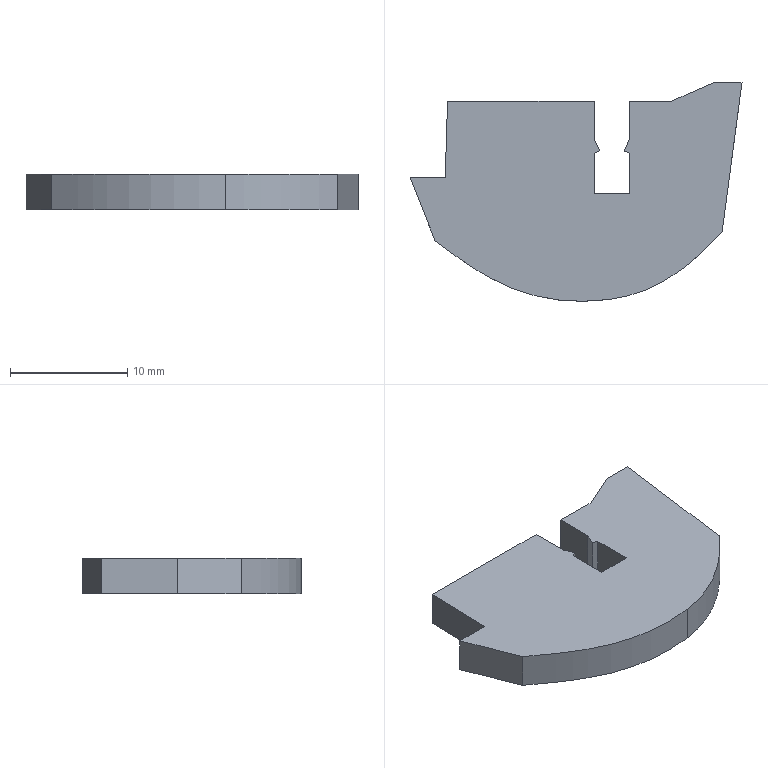Part | SolidWorks | features BaseBody 1 | 1 solid | 21 faces | box 28.291 x 18.638 x 3 mm | volume 1097 mm3 | plane 15 | spline 6
STEP:
#1=CARTESIAN_POINT('',(9.111,-14.247,-1.5));
#2=VERTEX_POINT('',#1);
#3=CARTESIAN_POINT('',(-0.4619,-19.968,-1.5));
#4=VERTEX_POINT('',#3);
#5=CARTESIAN_POINT('',(9.111,-14.247,-1.5));
#6=CARTESIAN_POINT('',(7.044,-16.596,-1.5));
#7=CARTESIAN_POINT('',(3.804,-19.425,-1.5));
#8=CARTESIAN_POINT('',(-0.4619,-19.968,-1.5));
#9=B_SPLINE_CURVE_WITH_KNOTS('',3,(#5,#6,#7,#8),.UNSPECIFIED.,.F.,.F.,(4,4),(0.9,1.),.UNSPECIFIED.);
#10=EDGE_CURVE('',#2,#4,#9,.T.);
#11=ORIENTED_EDGE('',*,*,#10,.T.);
#12=CARTESIAN_POINT('',(-15.322,-15.,-1.5));
#13=VERTEX_POINT('',#12);
#14=CARTESIAN_POINT('',(-0.4619,-19.968,-1.5));
#15=CARTESIAN_POINT('',(-7.402,-20.85,-1.5));
#16=CARTESIAN_POINT('',(-11.363,-17.925,-1.5));
#17=CARTESIAN_POINT('',(-15.322,-15.,-1.5));
#18=B_SPLINE_CURVE_WITH_KNOTS('',3,(#14,#15,#16,#17),.UNSPECIFIED.,.F.,.F.,(4,4),(0.,0.05),.UNSPECIFIED.);
#19=EDGE_CURVE('',#4,#13,#18,.T.);
#20=ORIENTED_EDGE('',*,*,#19,.T.);
#21=CARTESIAN_POINT('',(-17.475,-9.564,-1.5));
#22=VERTEX_POINT('',#21);
#23=CARTESIAN_POINT('',(-15.322,-15.,-1.5));
#24=CARTESIAN_POINT('',(-16.041,-13.188,-1.5));
#25=CARTESIAN_POINT('',(-16.758,-11.376,-1.5));
#26=CARTESIAN_POINT('',(-17.475,-9.564,-1.5));
#27=B_SPLINE_CURVE_WITH_KNOTS('',3,(#23,#24,#25,#26),.UNSPECIFIED.,.F.,.F.,(4,4),(0.05,0.1),.UNSPECIFIED.);
#28=EDGE_CURVE('',#13,#22,#27,.T.);
#29=ORIENTED_EDGE('',*,*,#28,.T.);
#30=CARTESIAN_POINT('',(-14.475,-9.564,-1.5));
#31=VERTEX_POINT('',#30);
#32=CARTESIAN_POINT('',(-17.475,-9.564,-1.5));
#33=DIRECTION('',(1.,0.,0.));
#34=VECTOR('',#33,1000.);
#35=LINE('',#32,#34);
#36=EDGE_CURVE('',#22,#31,#35,.T.);
#37=ORIENTED_EDGE('',*,*,#36,.T.);
#38=CARTESIAN_POINT('',(-14.277,-3.061,-1.5));
#39=VERTEX_POINT('',#38);
#40=CARTESIAN_POINT('',(-14.475,-9.564,-1.5));
#41=CARTESIAN_POINT('',(-14.393,-6.871,-1.5));
#42=CARTESIAN_POINT('',(-14.359,-5.755,-1.5));
#43=CARTESIAN_POINT('',(-14.277,-3.061,-1.5));
#44=B_SPLINE_CURVE_WITH_KNOTS('',3,(#40,#41,#42,#43),.UNSPECIFIED.,.F.,.F.,(4,4),(0.15,0.2),.UNSPECIFIED.);
#45=EDGE_CURVE('',#31,#39,#44,.T.);
#46=ORIENTED_EDGE('',*,*,#45,.T.);
#47=CARTESIAN_POINT('',(-1.772,-3.061,-1.5));
#48=VERTEX_POINT('',#47);
#49=CARTESIAN_POINT('',(-14.277,-3.061,-1.5));
#50=DIRECTION('',(1.,0.,0.));
#51=VECTOR('',#50,1000.);
#52=LINE('',#49,#51);
#53=EDGE_CURVE('',#39,#48,#52,.T.);
#54=ORIENTED_EDGE('',*,*,#53,.T.);
#55=CARTESIAN_POINT('',(-1.772,-6.322,-1.5));
#56=VERTEX_POINT('',#55);
#57=CARTESIAN_POINT('',(-1.772,-3.061,-1.5));
#58=DIRECTION('',(0.,-1.,0.));
#59=VECTOR('',#58,1000.);
#60=LINE('',#57,#59);
#61=EDGE_CURVE('',#48,#56,#60,.T.);
#62=ORIENTED_EDGE('',*,*,#61,.T.);
#63=CARTESIAN_POINT('',(-1.323,-7.28,-1.5));
#64=VERTEX_POINT('',#63);
#65=CARTESIAN_POINT('',(-1.772,-6.322,-1.5));
#66=DIRECTION('',(0.4242,-0.9056,0.));
#67=VECTOR('',#66,1000.);
#68=LINE('',#65,#67);
#69=EDGE_CURVE('',#56,#64,#68,.T.);
#70=ORIENTED_EDGE('',*,*,#69,.T.);
#71=CARTESIAN_POINT('',(-1.772,-7.511,-1.5));
#72=VERTEX_POINT('',#71);
#73=CARTESIAN_POINT('',(-1.323,-7.28,-1.5));
#74=DIRECTION('',(-0.8893,-0.4572,0.));
#75=VECTOR('',#74,1000.);
#76=LINE('',#73,#75);
#77=EDGE_CURVE('',#64,#72,#76,.T.);
#78=ORIENTED_EDGE('',*,*,#77,.T.);
#79=CARTESIAN_POINT('',(-1.772,-10.963,-1.5));
#80=VERTEX_POINT('',#79);
#81=CARTESIAN_POINT('',(-1.772,-7.511,-1.5));
#82=DIRECTION('',(0.,-1.,0.));
#83=VECTOR('',#82,1000.);
#84=LINE('',#81,#83);
#85=EDGE_CURVE('',#72,#80,#84,.T.);
#86=ORIENTED_EDGE('',*,*,#85,.T.);
#87=CARTESIAN_POINT('',(1.224,-10.963,-1.5));
#88=VERTEX_POINT('',#87);
#89=CARTESIAN_POINT('',(-1.772,-10.963,-1.5));
#90=DIRECTION('',(1.,0.,0.));
#91=VECTOR('',#90,1000.);
#92=LINE('',#89,#91);
#93=EDGE_CURVE('',#80,#88,#92,.T.);
#94=ORIENTED_EDGE('',*,*,#93,.T.);
#95=CARTESIAN_POINT('',(1.224,-7.511,-1.5));
#96=VERTEX_POINT('',#95);
#97=CARTESIAN_POINT('',(1.224,-10.963,-1.5));
#98=DIRECTION('',(0.,1.,0.));
#99=VECTOR('',#98,1000.);
#100=LINE('',#97,#99);
#101=EDGE_CURVE('',#88,#96,#100,.T.);
#102=ORIENTED_EDGE('',*,*,#101,.T.);
#103=CARTESIAN_POINT('',(0.7738,-7.315,-1.5));
#104=VERTEX_POINT('',#103);
#105=CARTESIAN_POINT('',(1.224,-7.511,-1.5));
#106=DIRECTION('',(-0.917,0.3989,0.));
#107=VECTOR('',#106,1000.);
#108=LINE('',#105,#107);
#109=EDGE_CURVE('',#96,#104,#108,.T.);
#110=ORIENTED_EDGE('',*,*,#109,.T.);
#111=CARTESIAN_POINT('',(1.224,-6.304,-1.5));
#112=VERTEX_POINT('',#111);
#113=CARTESIAN_POINT('',(0.7738,-7.315,-1.5));
#114=DIRECTION('',(0.4071,0.9134,0.));
#115=VECTOR('',#114,1000.);
#116=LINE('',#113,#115);
#117=EDGE_CURVE('',#104,#112,#116,.T.);
#118=ORIENTED_EDGE('',*,*,#117,.T.);
#119=CARTESIAN_POINT('',(1.224,-3.061,-1.5));
#120=VERTEX_POINT('',#119);
#121=CARTESIAN_POINT('',(1.224,-6.304,-1.5));
#122=DIRECTION('',(0.,1.,0.));
#123=VECTOR('',#122,1000.);
#124=LINE('',#121,#123);
#125=EDGE_CURVE('',#112,#120,#124,.T.);
#126=ORIENTED_EDGE('',*,*,#125,.T.);
#127=CARTESIAN_POINT('',(4.844,-3.061,-1.5));
#128=VERTEX_POINT('',#127);
#129=CARTESIAN_POINT('',(1.224,-3.061,-1.5));
#130=DIRECTION('',(1.,0.,0.));
#131=VECTOR('',#130,1000.);
#132=LINE('',#129,#131);
#133=EDGE_CURVE('',#120,#128,#132,.T.);
#134=ORIENTED_EDGE('',*,*,#133,.T.);
#135=CARTESIAN_POINT('',(8.366,-1.493,-1.5));
#136=VERTEX_POINT('',#135);
#137=CARTESIAN_POINT('',(4.844,-3.061,-1.5));
#138=DIRECTION('',(0.9136,0.4066,0.));
#139=VECTOR('',#138,1000.);
#140=LINE('',#137,#139);
#141=EDGE_CURVE('',#128,#136,#140,.T.);
#142=ORIENTED_EDGE('',*,*,#141,.T.);
#143=CARTESIAN_POINT('',(10.816,-1.489,-1.5));
#144=VERTEX_POINT('',#143);
#145=CARTESIAN_POINT('',(8.366,-1.493,-1.5));
#146=CARTESIAN_POINT('',(9.409,-1.491,-1.5));
#147=CARTESIAN_POINT('',(10.816,-1.489,-1.5));
#148=B_SPLINE_CURVE_WITH_KNOTS('',2,(#145,#146,#147),.UNSPECIFIED.,.F.,.F.,(3,3),(0.8,0.85),.UNSPECIFIED.);
#149=EDGE_CURVE('',#136,#144,#148,.T.);
#150=ORIENTED_EDGE('',*,*,#149,.T.);
#151=CARTESIAN_POINT('',(10.816,-1.489,-1.5));
#152=CARTESIAN_POINT('',(10.53,-3.621,-1.5));
#153=CARTESIAN_POINT('',(9.723,-9.669,-1.5));
#154=CARTESIAN_POINT('',(9.111,-14.247,-1.5));
#155=B_SPLINE_CURVE_WITH_KNOTS('',3,(#151,#152,#153,#154),.UNSPECIFIED.,.F.,.F.,(4,4),(0.85,0.9),.UNSPECIFIED.);
#156=EDGE_CURVE('',#144,#2,#155,.T.);
#157=ORIENTED_EDGE('',*,*,#156,.T.);
#158=EDGE_LOOP('',(#11,#20,#29,#37,#46,#54,#62,#70,#78,#86,#94,#102,#110,#118,#126,#134,#142,#150,#157));
#159=FACE_OUTER_BOUND('',#158,.T.);
#160=CARTESIAN_POINT('',(5.149,-17.785,-1.5));
#161=DIRECTION('',(0.,0.,1.));
#162=DIRECTION('',(1.,0.,0.));
#163=AXIS2_PLACEMENT_3D('',#160,#161,#162);
#164=PLANE('',#163);
#165=ADVANCED_FACE('',(#159),#164,.F.);
#166=CARTESIAN_POINT('',(9.111,-14.247,1.5));
#167=VERTEX_POINT('',#166);
#168=CARTESIAN_POINT('',(-0.4619,-19.968,1.5));
#169=VERTEX_POINT('',#168);
#170=CARTESIAN_POINT('',(9.111,-14.247,1.5));
#171=CARTESIAN_POINT('',(7.044,-16.596,1.5));
#172=CARTESIAN_POINT('',(3.804,-19.425,1.5));
#173=CARTESIAN_POINT('',(-0.4619,-19.968,1.5));
#174=B_SPLINE_CURVE_WITH_KNOTS('',3,(#170,#171,#172,#173),.UNSPECIFIED.,.F.,.F.,(4,4),(0.9,1.),.UNSPECIFIED.);
#175=EDGE_CURVE('',#167,#169,#174,.T.);
#176=ORIENTED_EDGE('',*,*,#175,.F.);
#177=CARTESIAN_POINT('',(10.816,-1.489,1.5));
#178=VERTEX_POINT('',#177);
#179=CARTESIAN_POINT('',(10.816,-1.489,1.5));
#180=CARTESIAN_POINT('',(10.53,-3.621,1.5));
#181=CARTESIAN_POINT('',(9.723,-9.669,1.5));
#182=CARTESIAN_POINT('',(9.111,-14.247,1.5));
#183=B_SPLINE_CURVE_WITH_KNOTS('',3,(#179,#180,#181,#182),.UNSPECIFIED.,.F.,.F.,(4,4),(0.85,0.9),.UNSPECIFIED.);
#184=EDGE_CURVE('',#178,#167,#183,.T.);
#185=ORIENTED_EDGE('',*,*,#184,.F.);
#186=CARTESIAN_POINT('',(8.366,-1.493,1.5));
#187=VERTEX_POINT('',#186);
#188=CARTESIAN_POINT('',(8.366,-1.493,1.5));
#189=CARTESIAN_POINT('',(9.409,-1.491,1.5));
#190=CARTESIAN_POINT('',(10.816,-1.489,1.5));
#191=B_SPLINE_CURVE_WITH_KNOTS('',2,(#188,#189,#190),.UNSPECIFIED.,.F.,.F.,(3,3),(0.8,0.85),.UNSPECIFIED.);
#192=EDGE_CURVE('',#187,#178,#191,.T.);
#193=ORIENTED_EDGE('',*,*,#192,.F.);
#194=CARTESIAN_POINT('',(4.844,-3.061,1.5));
#195=VERTEX_POINT('',#194);
#196=CARTESIAN_POINT('',(4.844,-3.061,1.5));
#197=DIRECTION('',(0.9136,0.4066,0.));
#198=VECTOR('',#197,1000.);
#199=LINE('',#196,#198);
#200=EDGE_CURVE('',#195,#187,#199,.T.);
#201=ORIENTED_EDGE('',*,*,#200,.F.);
#202=CARTESIAN_POINT('',(1.224,-3.061,1.5));
#203=VERTEX_POINT('',#202);
#204=CARTESIAN_POINT('',(1.224,-3.061,1.5));
#205=DIRECTION('',(1.,0.,0.));
#206=VECTOR('',#205,1000.);
#207=LINE('',#204,#206);
#208=EDGE_CURVE('',#203,#195,#207,.T.);
#209=ORIENTED_EDGE('',*,*,#208,.F.);
#210=CARTESIAN_POINT('',(1.224,-6.304,1.5));
#211=VERTEX_POINT('',#210);
#212=CARTESIAN_POINT('',(1.224,-6.304,1.5));
#213=DIRECTION('',(0.,1.,0.));
#214=VECTOR('',#213,1000.);
#215=LINE('',#212,#214);
#216=EDGE_CURVE('',#211,#203,#215,.T.);
#217=ORIENTED_EDGE('',*,*,#216,.F.);
#218=CARTESIAN_POINT('',(0.7738,-7.315,1.5));
#219=VERTEX_POINT('',#218);
#220=CARTESIAN_POINT('',(0.7738,-7.315,1.5));
#221=DIRECTION('',(0.4071,0.9134,0.));
#222=VECTOR('',#221,1000.);
#223=LINE('',#220,#222);
#224=EDGE_CURVE('',#219,#211,#223,.T.);
#225=ORIENTED_EDGE('',*,*,#224,.F.);
#226=CARTESIAN_POINT('',(1.224,-7.511,1.5));
#227=VERTEX_POINT('',#226);
#228=CARTESIAN_POINT('',(1.224,-7.511,1.5));
#229=DIRECTION('',(-0.917,0.3989,0.));
#230=VECTOR('',#229,1000.);
#231=LINE('',#228,#230);
#232=EDGE_CURVE('',#227,#219,#231,.T.);
#233=ORIENTED_EDGE('',*,*,#232,.F.);
#234=CARTESIAN_POINT('',(1.224,-10.963,1.5));
#235=VERTEX_POINT('',#234);
#236=CARTESIAN_POINT('',(1.224,-10.963,1.5));
#237=DIRECTION('',(0.,1.,0.));
#238=VECTOR('',#237,1000.);
#239=LINE('',#236,#238);
#240=EDGE_CURVE('',#235,#227,#239,.T.);
#241=ORIENTED_EDGE('',*,*,#240,.F.);
#242=CARTESIAN_POINT('',(-1.772,-10.963,1.5));
#243=VERTEX_POINT('',#242);
#244=CARTESIAN_POINT('',(-1.772,-10.963,1.5));
#245=DIRECTION('',(1.,0.,0.));
#246=VECTOR('',#245,1000.);
#247=LINE('',#244,#246);
#248=EDGE_CURVE('',#243,#235,#247,.T.);
#249=ORIENTED_EDGE('',*,*,#248,.F.);
#250=CARTESIAN_POINT('',(-1.772,-7.511,1.5));
#251=VERTEX_POINT('',#250);
#252=CARTESIAN_POINT('',(-1.772,-7.511,1.5));
#253=DIRECTION('',(0.,-1.,0.));
#254=VECTOR('',#253,1000.);
#255=LINE('',#252,#254);
#256=EDGE_CURVE('',#251,#243,#255,.T.);
#257=ORIENTED_EDGE('',*,*,#256,.F.);
#258=CARTESIAN_POINT('',(-1.323,-7.28,1.5));
#259=VERTEX_POINT('',#258);
#260=CARTESIAN_POINT('',(-1.323,-7.28,1.5));
#261=DIRECTION('',(-0.8893,-0.4572,0.));
#262=VECTOR('',#261,1000.);
#263=LINE('',#260,#262);
#264=EDGE_CURVE('',#259,#251,#263,.T.);
#265=ORIENTED_EDGE('',*,*,#264,.F.);
#266=CARTESIAN_POINT('',(-1.772,-6.322,1.5));
#267=VERTEX_POINT('',#266);
#268=CARTESIAN_POINT('',(-1.772,-6.322,1.5));
#269=DIRECTION('',(0.4242,-0.9056,0.));
#270=VECTOR('',#269,1000.);
#271=LINE('',#268,#270);
#272=EDGE_CURVE('',#267,#259,#271,.T.);
#273=ORIENTED_EDGE('',*,*,#272,.F.);
#274=CARTESIAN_POINT('',(-1.772,-3.061,1.5));
#275=VERTEX_POINT('',#274);
#276=CARTESIAN_POINT('',(-1.772,-3.061,1.5));
#277=DIRECTION('',(0.,-1.,0.));
#278=VECTOR('',#277,1000.);
#279=LINE('',#276,#278);
#280=EDGE_CURVE('',#275,#267,#279,.T.);
#281=ORIENTED_EDGE('',*,*,#280,.F.);
#282=CARTESIAN_POINT('',(-14.277,-3.061,1.5));
#283=VERTEX_POINT('',#282);
#284=CARTESIAN_POINT('',(-14.277,-3.061,1.5));
#285=DIRECTION('',(1.,0.,0.));
#286=VECTOR('',#285,1000.);
#287=LINE('',#284,#286);
#288=EDGE_CURVE('',#283,#275,#287,.T.);
#289=ORIENTED_EDGE('',*,*,#288,.F.);
#290=CARTESIAN_POINT('',(-14.475,-9.564,1.5));
#291=VERTEX_POINT('',#290);
#292=CARTESIAN_POINT('',(-14.475,-9.564,1.5));
#293=CARTESIAN_POINT('',(-14.393,-6.871,1.5));
#294=CARTESIAN_POINT('',(-14.359,-5.755,1.5));
#295=CARTESIAN_POINT('',(-14.277,-3.061,1.5));
#296=B_SPLINE_CURVE_WITH_KNOTS('',3,(#292,#293,#294,#295),.UNSPECIFIED.,.F.,.F.,(4,4),(0.15,0.2),.UNSPECIFIED.);
#297=EDGE_CURVE('',#291,#283,#296,.T.);
#298=ORIENTED_EDGE('',*,*,#297,.F.);
#299=CARTESIAN_POINT('',(-17.475,-9.564,1.5));
#300=VERTEX_POINT('',#299);
#301=CARTESIAN_POINT('',(-17.475,-9.564,1.5));
#302=DIRECTION('',(1.,0.,0.));
#303=VECTOR('',#302,1000.);
#304=LINE('',#301,#303);
#305=EDGE_CURVE('',#300,#291,#304,.T.);
#306=ORIENTED_EDGE('',*,*,#305,.F.);
#307=CARTESIAN_POINT('',(-15.322,-15.,1.5));
#308=VERTEX_POINT('',#307);
#309=CARTESIAN_POINT('',(-15.322,-15.,1.5));
#310=CARTESIAN_POINT('',(-16.041,-13.188,1.5));
#311=CARTESIAN_POINT('',(-16.758,-11.376,1.5));
#312=CARTESIAN_POINT('',(-17.475,-9.564,1.5));
#313=B_SPLINE_CURVE_WITH_KNOTS('',3,(#309,#310,#311,#312),.UNSPECIFIED.,.F.,.F.,(4,4),(0.05,0.1),.UNSPECIFIED.);
#314=EDGE_CURVE('',#308,#300,#313,.T.);
#315=ORIENTED_EDGE('',*,*,#314,.F.);
#316=CARTESIAN_POINT('',(-0.4619,-19.968,1.5));
#317=CARTESIAN_POINT('',(-7.402,-20.85,1.5));
#318=CARTESIAN_POINT('',(-11.363,-17.925,1.5));
#319=CARTESIAN_POINT('',(-15.322,-15.,1.5));
#320=B_SPLINE_CURVE_WITH_KNOTS('',3,(#316,#317,#318,#319),.UNSPECIFIED.,.F.,.F.,(4,4),(0.,0.05),.UNSPECIFIED.);
#321=EDGE_CURVE('',#169,#308,#320,.T.);
#322=ORIENTED_EDGE('',*,*,#321,.F.);
#323=EDGE_LOOP('',(#176,#185,#193,#201,#209,#217,#225,#233,#241,#249,#257,#265,#273,#281,#289,#298,#306,#315,#322));
#324=FACE_OUTER_BOUND('',#323,.T.);
#325=CARTESIAN_POINT('',(5.149,-17.785,1.5));
#326=DIRECTION('',(0.,0.,1.));
#327=DIRECTION('',(1.,0.,0.));
#328=AXIS2_PLACEMENT_3D('',#325,#326,#327);
#329=PLANE('',#328);
#330=ADVANCED_FACE('',(#324),#329,.T.);
#331=ORIENTED_EDGE('',*,*,#19,.F.);
#332=CARTESIAN_POINT('',(-0.4619,-19.968,1.5));
#333=DIRECTION('',(0.,0.,-1.));
#334=VECTOR('',#333,1000.);
#335=LINE('',#332,#334);
#336=EDGE_CURVE('',#169,#4,#335,.T.);
#337=ORIENTED_EDGE('',*,*,#336,.F.);
#338=ORIENTED_EDGE('',*,*,#321,.T.);
#339=CARTESIAN_POINT('',(-15.322,-15.,1.5));
#340=DIRECTION('',(0.,0.,-1.));
#341=VECTOR('',#340,1000.);
#342=LINE('',#339,#341);
#343=EDGE_CURVE('',#308,#13,#342,.T.);
#344=ORIENTED_EDGE('',*,*,#343,.T.);
#345=EDGE_LOOP('',(#331,#337,#338,#344));
#346=FACE_OUTER_BOUND('',#345,.T.);
#347=CARTESIAN_POINT('',(-0.4619,-19.968,1.5));
#348=CARTESIAN_POINT('',(-0.4619,-19.968,-1.5));
#349=CARTESIAN_POINT('',(-7.402,-20.85,1.5));
#350=CARTESIAN_POINT('',(-7.402,-20.85,-1.5));
#351=CARTESIAN_POINT('',(-11.363,-17.925,1.5));
#352=CARTESIAN_POINT('',(-11.363,-17.925,-1.5));
#353=CARTESIAN_POINT('',(-15.322,-15.,1.5));
#354=CARTESIAN_POINT('',(-15.322,-15.,-1.5));
#355=B_SPLINE_SURFACE_WITH_KNOTS('',3,1,((#347,#348),(#349,#350),(#351,#352),(#353,#354)),.UNSPECIFIED.,.F.,.F.,.F.,(4,4),(2,2),(0.,0.05),(0.,1.),.UNSPECIFIED.);
#356=ADVANCED_FACE('',(#346),#355,.T.);
#357=ORIENTED_EDGE('',*,*,#28,.F.);
#358=ORIENTED_EDGE('',*,*,#343,.F.);
#359=ORIENTED_EDGE('',*,*,#314,.T.);
#360=CARTESIAN_POINT('',(-17.475,-9.564,1.5));
#361=DIRECTION('',(0.,0.,-1.));
#362=VECTOR('',#361,1000.);
#363=LINE('',#360,#362);
#364=EDGE_CURVE('',#300,#22,#363,.T.);
#365=ORIENTED_EDGE('',*,*,#364,.T.);
#366=EDGE_LOOP('',(#357,#358,#359,#365));
#367=FACE_OUTER_BOUND('',#366,.T.);
#368=CARTESIAN_POINT('',(-15.322,-15.,1.5));
#369=CARTESIAN_POINT('',(-15.322,-15.,-1.5));
#370=CARTESIAN_POINT('',(-16.041,-13.188,1.5));
#371=CARTESIAN_POINT('',(-16.041,-13.188,-1.5));
#372=CARTESIAN_POINT('',(-16.758,-11.376,1.5));
#373=CARTESIAN_POINT('',(-16.758,-11.376,-1.5));
#374=CARTESIAN_POINT('',(-17.475,-9.564,1.5));
#375=CARTESIAN_POINT('',(-17.475,-9.564,-1.5));
#376=B_SPLINE_SURFACE_WITH_KNOTS('',3,1,((#368,#369),(#370,#371),(#372,#373),(#374,#375)),.UNSPECIFIED.,.F.,.F.,.F.,(4,4),(2,2),(0.05,0.1),(0.,1.),.UNSPECIFIED.);
#377=ADVANCED_FACE('',(#367),#376,.T.);
#378=ORIENTED_EDGE('',*,*,#36,.F.);
#379=ORIENTED_EDGE('',*,*,#364,.F.);
#380=ORIENTED_EDGE('',*,*,#305,.T.);
#381=CARTESIAN_POINT('',(-14.475,-9.564,1.5));
#382=DIRECTION('',(0.,0.,-1.));
#383=VECTOR('',#382,1000.);
#384=LINE('',#381,#383);
#385=EDGE_CURVE('',#291,#31,#384,.T.);
#386=ORIENTED_EDGE('',*,*,#385,.T.);
#387=EDGE_LOOP('',(#378,#379,#380,#386));
#388=FACE_OUTER_BOUND('',#387,.T.);
#389=CARTESIAN_POINT('',(-17.475,-9.564,1.5));
#390=DIRECTION('',(0.,1.,0.));
#391=DIRECTION('',(1.,0.,0.));
#392=AXIS2_PLACEMENT_3D('',#389,#390,#391);
#393=PLANE('',#392);
#394=ADVANCED_FACE('',(#388),#393,.T.);
#395=ORIENTED_EDGE('',*,*,#45,.F.);
#396=ORIENTED_EDGE('',*,*,#385,.F.);
#397=ORIENTED_EDGE('',*,*,#297,.T.);
#398=CARTESIAN_POINT('',(-14.277,-3.061,1.5));
#399=DIRECTION('',(0.,0.,-1.));
#400=VECTOR('',#399,1000.);
#401=LINE('',#398,#400);
#402=EDGE_CURVE('',#283,#39,#401,.T.);
#403=ORIENTED_EDGE('',*,*,#402,.T.);
#404=EDGE_LOOP('',(#395,#396,#397,#403));
#405=FACE_OUTER_BOUND('',#404,.T.);
#406=CARTESIAN_POINT('',(-14.475,-9.564,1.5));
#407=CARTESIAN_POINT('',(-14.475,-9.564,-1.5));
#408=CARTESIAN_POINT('',(-14.393,-6.871,1.5));
#409=CARTESIAN_POINT('',(-14.393,-6.871,-1.5));
#410=CARTESIAN_POINT('',(-14.359,-5.755,1.5));
#411=CARTESIAN_POINT('',(-14.359,-5.755,-1.5));
#412=CARTESIAN_POINT('',(-14.277,-3.061,1.5));
#413=CARTESIAN_POINT('',(-14.277,-3.061,-1.5));
#414=B_SPLINE_SURFACE_WITH_KNOTS('',3,1,((#406,#407),(#408,#409),(#410,#411),(#412,#413)),.UNSPECIFIED.,.F.,.F.,.F.,(4,4),(2,2),(0.15,0.2),(0.,1.),.UNSPECIFIED.);
#415=ADVANCED_FACE('',(#405),#414,.T.);
#416=ORIENTED_EDGE('',*,*,#53,.F.);
#417=ORIENTED_EDGE('',*,*,#402,.F.);
#418=ORIENTED_EDGE('',*,*,#288,.T.);
#419=CARTESIAN_POINT('',(-1.772,-3.061,1.5));
#420=DIRECTION('',(0.,0.,-1.));
#421=VECTOR('',#420,1000.);
#422=LINE('',#419,#421);
#423=EDGE_CURVE('',#275,#48,#422,.T.);
#424=ORIENTED_EDGE('',*,*,#423,.T.);
#425=EDGE_LOOP('',(#416,#417,#418,#424));
#426=FACE_OUTER_BOUND('',#425,.T.);
#427=CARTESIAN_POINT('',(-14.277,-3.061,1.5));
#428=DIRECTION('',(0.,1.,0.));
#429=DIRECTION('',(1.,0.,0.));
#430=AXIS2_PLACEMENT_3D('',#427,#428,#429);
#431=PLANE('',#430);
#432=ADVANCED_FACE('',(#426),#431,.T.);
#433=ORIENTED_EDGE('',*,*,#61,.F.);
#434=ORIENTED_EDGE('',*,*,#423,.F.);
#435=ORIENTED_EDGE('',*,*,#280,.T.);
#436=CARTESIAN_POINT('',(-1.772,-6.322,1.5));
#437=DIRECTION('',(0.,0.,-1.));
#438=VECTOR('',#437,1000.);
#439=LINE('',#436,#438);
#440=EDGE_CURVE('',#267,#56,#439,.T.);
#441=ORIENTED_EDGE('',*,*,#440,.T.);
#442=EDGE_LOOP('',(#433,#434,#435,#441));
#443=FACE_OUTER_BOUND('',#442,.T.);
#444=CARTESIAN_POINT('',(-1.772,-3.061,1.5));
#445=DIRECTION('',(1.,0.,0.));
#446=DIRECTION('',(0.,1.,0.));
#447=AXIS2_PLACEMENT_3D('',#444,#445,#446);
#448=PLANE('',#447);
#449=ADVANCED_FACE('',(#443),#448,.T.);
#450=ORIENTED_EDGE('',*,*,#69,.F.);
#451=ORIENTED_EDGE('',*,*,#440,.F.);
#452=ORIENTED_EDGE('',*,*,#272,.T.);
#453=CARTESIAN_POINT('',(-1.323,-7.28,1.5));
#454=DIRECTION('',(0.,0.,-1.));
#455=VECTOR('',#454,1000.);
#456=LINE('',#453,#455);
#457=EDGE_CURVE('',#259,#64,#456,.T.);
#458=ORIENTED_EDGE('',*,*,#457,.T.);
#459=EDGE_LOOP('',(#450,#451,#452,#458));
#460=FACE_OUTER_BOUND('',#459,.T.);
#461=CARTESIAN_POINT('',(-1.772,-6.322,1.5));
#462=DIRECTION('',(0.9056,0.4242,0.));
#463=DIRECTION('',(0.,0.,-1.));
#464=AXIS2_PLACEMENT_3D('',#461,#462,#463);
#465=PLANE('',#464);
#466=ADVANCED_FACE('',(#460),#465,.T.);
#467=ORIENTED_EDGE('',*,*,#77,.F.);
#468=ORIENTED_EDGE('',*,*,#457,.F.);
#469=ORIENTED_EDGE('',*,*,#264,.T.);
#470=CARTESIAN_POINT('',(-1.772,-7.511,1.5));
#471=DIRECTION('',(0.,0.,-1.));
#472=VECTOR('',#471,1000.);
#473=LINE('',#470,#472);
#474=EDGE_CURVE('',#251,#72,#473,.T.);
#475=ORIENTED_EDGE('',*,*,#474,.T.);
#476=EDGE_LOOP('',(#467,#468,#469,#475));
#477=FACE_OUTER_BOUND('',#476,.T.);
#478=CARTESIAN_POINT('',(-1.323,-7.28,1.5));
#479=DIRECTION('',(0.4572,-0.8893,0.));
#480=DIRECTION('',(0.,0.,-1.));
#481=AXIS2_PLACEMENT_3D('',#478,#479,#480);
#482=PLANE('',#481);
#483=ADVANCED_FACE('',(#477),#482,.T.);
#484=ORIENTED_EDGE('',*,*,#85,.F.);
#485=ORIENTED_EDGE('',*,*,#474,.F.);
#486=ORIENTED_EDGE('',*,*,#256,.T.);
#487=CARTESIAN_POINT('',(-1.772,-10.963,1.5));
#488=DIRECTION('',(0.,0.,-1.));
#489=VECTOR('',#488,1000.);
#490=LINE('',#487,#489);
#491=EDGE_CURVE('',#243,#80,#490,.T.);
#492=ORIENTED_EDGE('',*,*,#491,.T.);
#493=EDGE_LOOP('',(#484,#485,#486,#492));
#494=FACE_OUTER_BOUND('',#493,.T.);
#495=CARTESIAN_POINT('',(-1.772,-7.511,1.5));
#496=DIRECTION('',(1.,0.,0.));
#497=DIRECTION('',(0.,1.,0.));
#498=AXIS2_PLACEMENT_3D('',#495,#496,#497);
#499=PLANE('',#498);
#500=ADVANCED_FACE('',(#494),#499,.T.);
#501=ORIENTED_EDGE('',*,*,#93,.F.);
#502=ORIENTED_EDGE('',*,*,#491,.F.);
#503=ORIENTED_EDGE('',*,*,#248,.T.);
#504=CARTESIAN_POINT('',(1.224,-10.963,1.5));
#505=DIRECTION('',(0.,0.,-1.));
#506=VECTOR('',#505,1000.);
#507=LINE('',#504,#506);
#508=EDGE_CURVE('',#235,#88,#507,.T.);
#509=ORIENTED_EDGE('',*,*,#508,.T.);
#510=EDGE_LOOP('',(#501,#502,#503,#509));
#511=FACE_OUTER_BOUND('',#510,.T.);
#512=CARTESIAN_POINT('',(-1.772,-10.963,1.5));
#513=DIRECTION('',(0.,1.,0.));
#514=DIRECTION('',(1.,0.,0.));
#515=AXIS2_PLACEMENT_3D('',#512,#513,#514);
#516=PLANE('',#515);
#517=ADVANCED_FACE('',(#511),#516,.T.);
#518=ORIENTED_EDGE('',*,*,#101,.F.);
#519=ORIENTED_EDGE('',*,*,#508,.F.);
#520=ORIENTED_EDGE('',*,*,#240,.T.);
#521=CARTESIAN_POINT('',(1.224,-7.511,1.5));
#522=DIRECTION('',(0.,0.,-1.));
#523=VECTOR('',#522,1000.);
#524=LINE('',#521,#523);
#525=EDGE_CURVE('',#227,#96,#524,.T.);
#526=ORIENTED_EDGE('',*,*,#525,.T.);
#527=EDGE_LOOP('',(#518,#519,#520,#526));
#528=FACE_OUTER_BOUND('',#527,.T.);
#529=CARTESIAN_POINT('',(1.224,-10.963,1.5));
#530=DIRECTION('',(-1.,0.,0.));
#531=DIRECTION('',(0.,0.,1.));
#532=AXIS2_PLACEMENT_3D('',#529,#530,#531);
#533=PLANE('',#532);
#534=ADVANCED_FACE('',(#528),#533,.T.);
#535=ORIENTED_EDGE('',*,*,#109,.F.);
#536=ORIENTED_EDGE('',*,*,#525,.F.);
#537=ORIENTED_EDGE('',*,*,#232,.T.);
#538=CARTESIAN_POINT('',(0.7738,-7.315,1.5));
#539=DIRECTION('',(0.,0.,-1.));
#540=VECTOR('',#539,1000.);
#541=LINE('',#538,#540);
#542=EDGE_CURVE('',#219,#104,#541,.T.);
#543=ORIENTED_EDGE('',*,*,#542,.T.);
#544=EDGE_LOOP('',(#535,#536,#537,#543));
#545=FACE_OUTER_BOUND('',#544,.T.);
#546=CARTESIAN_POINT('',(1.224,-7.511,1.5));
#547=DIRECTION('',(-0.3989,-0.917,0.));
#548=DIRECTION('',(-0.917,0.3989,0.));
#549=AXIS2_PLACEMENT_3D('',#546,#547,#548);
#550=PLANE('',#549);
#551=ADVANCED_FACE('',(#545),#550,.T.);
#552=ORIENTED_EDGE('',*,*,#117,.F.);
#553=ORIENTED_EDGE('',*,*,#542,.F.);
#554=ORIENTED_EDGE('',*,*,#224,.T.);
#555=CARTESIAN_POINT('',(1.224,-6.304,1.5));
#556=DIRECTION('',(0.,0.,-1.));
#557=VECTOR('',#556,1000.);
#558=LINE('',#555,#557);
#559=EDGE_CURVE('',#211,#112,#558,.T.);
#560=ORIENTED_EDGE('',*,*,#559,.T.);
#561=EDGE_LOOP('',(#552,#553,#554,#560));
#562=FACE_OUTER_BOUND('',#561,.T.);
#563=CARTESIAN_POINT('',(0.7738,-7.315,1.5));
#564=DIRECTION('',(-0.9134,0.4071,0.));
#565=DIRECTION('',(0.,0.,1.));
#566=AXIS2_PLACEMENT_3D('',#563,#564,#565);
#567=PLANE('',#566);
#568=ADVANCED_FACE('',(#562),#567,.T.);
#569=ORIENTED_EDGE('',*,*,#125,.F.);
#570=ORIENTED_EDGE('',*,*,#559,.F.);
#571=ORIENTED_EDGE('',*,*,#216,.T.);
#572=CARTESIAN_POINT('',(1.224,-3.061,1.5));
#573=DIRECTION('',(0.,0.,-1.));
#574=VECTOR('',#573,1000.);
#575=LINE('',#572,#574);
#576=EDGE_CURVE('',#203,#120,#575,.T.);
#577=ORIENTED_EDGE('',*,*,#576,.T.);
#578=EDGE_LOOP('',(#569,#570,#571,#577));
#579=FACE_OUTER_BOUND('',#578,.T.);
#580=CARTESIAN_POINT('',(1.224,-6.304,1.5));
#581=DIRECTION('',(-1.,0.,0.));
#582=DIRECTION('',(0.,0.,1.));
#583=AXIS2_PLACEMENT_3D('',#580,#581,#582);
#584=PLANE('',#583);
#585=ADVANCED_FACE('',(#579),#584,.T.);
#586=ORIENTED_EDGE('',*,*,#133,.F.);
#587=ORIENTED_EDGE('',*,*,#576,.F.);
#588=ORIENTED_EDGE('',*,*,#208,.T.);
#589=CARTESIAN_POINT('',(4.844,-3.061,1.5));
#590=DIRECTION('',(0.,0.,-1.));
#591=VECTOR('',#590,1000.);
#592=LINE('',#589,#591);
#593=EDGE_CURVE('',#195,#128,#592,.T.);
#594=ORIENTED_EDGE('',*,*,#593,.T.);
#595=EDGE_LOOP('',(#586,#587,#588,#594));
#596=FACE_OUTER_BOUND('',#595,.T.);
#597=CARTESIAN_POINT('',(1.224,-3.061,1.5));
#598=DIRECTION('',(0.,1.,0.));
#599=DIRECTION('',(1.,0.,0.));
#600=AXIS2_PLACEMENT_3D('',#597,#598,#599);
#601=PLANE('',#600);
#602=ADVANCED_FACE('',(#596),#601,.T.);
#603=ORIENTED_EDGE('',*,*,#141,.F.);
#604=ORIENTED_EDGE('',*,*,#593,.F.);
#605=ORIENTED_EDGE('',*,*,#200,.T.);
#606=CARTESIAN_POINT('',(8.366,-1.493,1.5));
#607=DIRECTION('',(0.,0.,-1.));
#608=VECTOR('',#607,1000.);
#609=LINE('',#606,#608);
#610=EDGE_CURVE('',#187,#136,#609,.T.);
#611=ORIENTED_EDGE('',*,*,#610,.T.);
#612=EDGE_LOOP('',(#603,#604,#605,#611));
#613=FACE_OUTER_BOUND('',#612,.T.);
#614=CARTESIAN_POINT('',(4.844,-3.061,1.5));
#615=DIRECTION('',(-0.4066,0.9136,0.));
#616=DIRECTION('',(0.,0.,1.));
#617=AXIS2_PLACEMENT_3D('',#614,#615,#616);
#618=PLANE('',#617);
#619=ADVANCED_FACE('',(#613),#618,.T.);
#620=ORIENTED_EDGE('',*,*,#149,.F.);
#621=ORIENTED_EDGE('',*,*,#610,.F.);
#622=ORIENTED_EDGE('',*,*,#192,.T.);
#623=CARTESIAN_POINT('',(10.816,-1.489,1.5));
#624=DIRECTION('',(0.,0.,-1.));
#625=VECTOR('',#624,1000.);
#626=LINE('',#623,#625);
#627=EDGE_CURVE('',#178,#144,#626,.T.);
#628=ORIENTED_EDGE('',*,*,#627,.T.);
#629=EDGE_LOOP('',(#620,#621,#622,#628));
#630=FACE_OUTER_BOUND('',#629,.T.);
#631=CARTESIAN_POINT('',(8.366,-1.493,1.5));
#632=CARTESIAN_POINT('',(8.366,-1.493,-1.5));
#633=CARTESIAN_POINT('',(9.409,-1.491,1.5));
#634=CARTESIAN_POINT('',(9.409,-1.491,-1.5));
#635=CARTESIAN_POINT('',(10.816,-1.489,1.5));
#636=CARTESIAN_POINT('',(10.816,-1.489,-1.5));
#637=B_SPLINE_SURFACE_WITH_KNOTS('',2,1,((#631,#632),(#633,#634),(#635,#636)),.UNSPECIFIED.,.F.,.F.,.F.,(3,3),(2,2),(0.8,0.85),(0.,1.),.UNSPECIFIED.);
#638=ADVANCED_FACE('',(#630),#637,.T.);
#639=ORIENTED_EDGE('',*,*,#156,.F.);
#640=ORIENTED_EDGE('',*,*,#627,.F.);
#641=ORIENTED_EDGE('',*,*,#184,.T.);
#642=CARTESIAN_POINT('',(9.111,-14.247,1.5));
#643=DIRECTION('',(0.,0.,-1.));
#644=VECTOR('',#643,1000.);
#645=LINE('',#642,#644);
#646=EDGE_CURVE('',#167,#2,#645,.T.);
#647=ORIENTED_EDGE('',*,*,#646,.T.);
#648=EDGE_LOOP('',(#639,#640,#641,#647));
#649=FACE_OUTER_BOUND('',#648,.T.);
#650=CARTESIAN_POINT('',(10.816,-1.489,1.5));
#651=CARTESIAN_POINT('',(10.816,-1.489,-1.5));
#652=CARTESIAN_POINT('',(10.53,-3.621,1.5));
#653=CARTESIAN_POINT('',(10.53,-3.621,-1.5));
#654=CARTESIAN_POINT('',(9.723,-9.669,1.5));
#655=CARTESIAN_POINT('',(9.723,-9.669,-1.5));
#656=CARTESIAN_POINT('',(9.111,-14.247,1.5));
#657=CARTESIAN_POINT('',(9.111,-14.247,-1.5));
#658=B_SPLINE_SURFACE_WITH_KNOTS('',3,1,((#650,#651),(#652,#653),(#654,#655),(#656,#657)),.UNSPECIFIED.,.F.,.F.,.F.,(4,4),(2,2),(0.85,0.9),(0.,1.),.UNSPECIFIED.);
#659=ADVANCED_FACE('',(#649),#658,.T.);
#660=ORIENTED_EDGE('',*,*,#10,.F.);
#661=ORIENTED_EDGE('',*,*,#646,.F.);
#662=ORIENTED_EDGE('',*,*,#175,.T.);
#663=ORIENTED_EDGE('',*,*,#336,.T.);
#664=EDGE_LOOP('',(#660,#661,#662,#663));
#665=FACE_OUTER_BOUND('',#664,.T.);
#666=CARTESIAN_POINT('',(9.111,-14.247,1.5));
#667=CARTESIAN_POINT('',(9.111,-14.247,-1.5));
#668=CARTESIAN_POINT('',(7.044,-16.596,1.5));
#669=CARTESIAN_POINT('',(7.044,-16.596,-1.5));
#670=CARTESIAN_POINT('',(3.804,-19.425,1.5));
#671=CARTESIAN_POINT('',(3.804,-19.425,-1.5));
#672=CARTESIAN_POINT('',(-0.4619,-19.968,1.5));
#673=CARTESIAN_POINT('',(-0.4619,-19.968,-1.5));
#674=B_SPLINE_SURFACE_WITH_KNOTS('',3,1,((#666,#667),(#668,#669),(#670,#671),(#672,#673)),.UNSPECIFIED.,.F.,.F.,.F.,(4,4),(2,2),(0.9,1.),(0.,1.),.UNSPECIFIED.);
#675=ADVANCED_FACE('',(#665),#674,.T.);
#676=CLOSED_SHELL('',(#165,#330,#356,#377,#394,#415,#432,#449,#466,#483,#500,#517,#534,#551,#568,#585,#602,#619,#638,#659,#675));
#677=MANIFOLD_SOLID_BREP('',#676);
#678=CARTESIAN_POINT('',(0.,0.,0.));
#679=DIRECTION('',(0.,0.,1.));
#680=DIRECTION('',(1.,0.,0.));
#681=AXIS2_PLACEMENT_3D('',#678,#679,#680);
#682=(LENGTH_UNIT()NAMED_UNIT(*)SI_UNIT(.MILLI.,.METRE.));
#683=UNCERTAINTY_MEASURE_WITH_UNIT(LENGTH_MEASURE(0.00001),#682,'','');
#684=(NAMED_UNIT(*)PLANE_ANGLE_UNIT()SI_UNIT($,.RADIAN.));
#685=(NAMED_UNIT(*)SI_UNIT($,.STERADIAN.)SOLID_ANGLE_UNIT());
#686=(GEOMETRIC_REPRESENTATION_CONTEXT(3)GLOBAL_UNCERTAINTY_ASSIGNED_CONTEXT((#683))GLOBAL_UNIT_ASSIGNED_CONTEXT((#682,#684,#685))REPRESENTATION_CONTEXT('',''));
#687=ADVANCED_BREP_SHAPE_REPRESENTATION('',(#677,#681),#686);